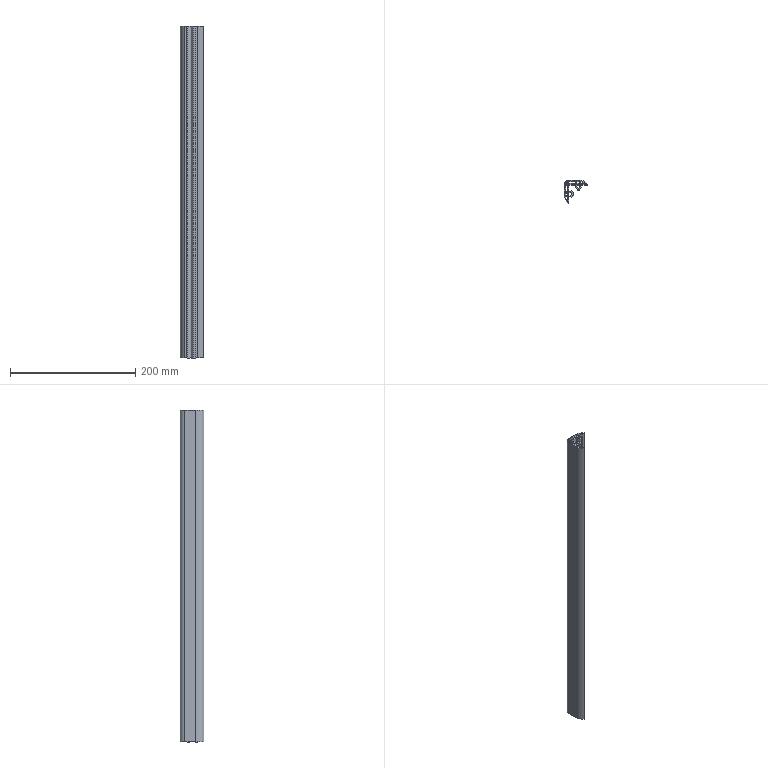Part | SolidWorks | features BaseBody 1, MoveFace 1 | 1 solid | 64 faces | box 37 x 37 x 530 mm | volume 171468 mm3 | plane 54 | cylinder 10 | commonest cylinder face diameters 20 x4 30 x4 11.068 x1 14 x1